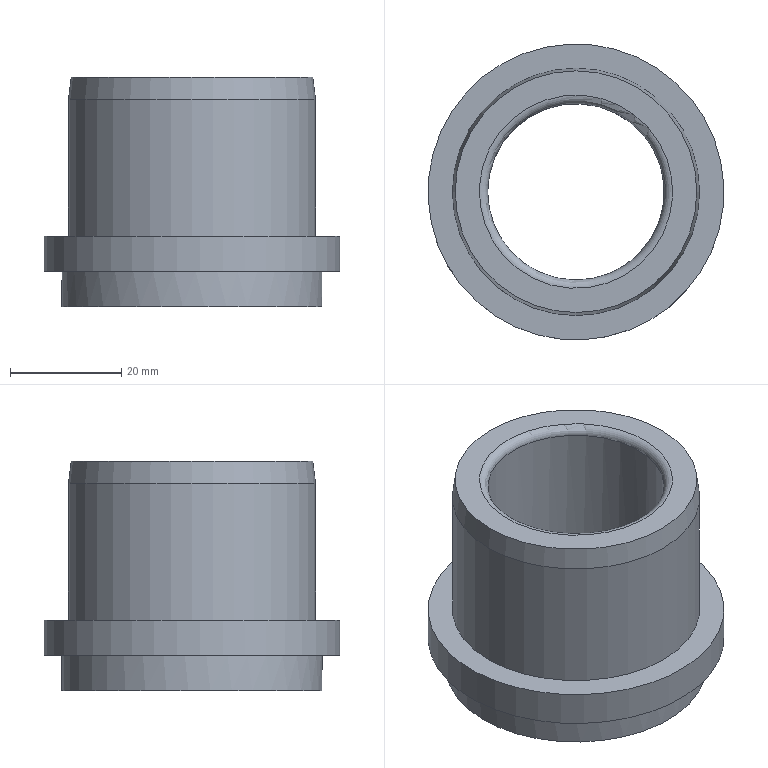Part | STEP file | 1_id1062_x_t | 1 solid | 11 faces | box 53.213 x 53.213 x 41.275 mm | volume 36326 mm3 | plane 4 | cylinder 4 | torus 2 | cone 1 | commonest cylinder face diameters 31.75 x1 44.45 x1 46.812 x1 53.213 x1
STEP:
#1=CARTESIAN_POINT('',(0.,0.,0.));
#2=DIRECTION('',(0.,0.,1.));
#3=DIRECTION('',(1.,0.,0.));
#4=AXIS2_PLACEMENT_3D('',#1,#2,#3);
#5=CARTESIAN_POINT('',(881.739,298.363,118.685));
#6=VERTEX_POINT('',#5);
#7=CARTESIAN_POINT('',(862.925,287.5,118.685));
#8=DIRECTION('',(0.,0.,1.));
#9=DIRECTION('',(0.866,0.5,0.));
#10=AXIS2_PLACEMENT_3D('',#7,#8,#9);
#11=CIRCLE('',#10,21.725);
#12=CARTESIAN_POINT('',(845.604,277.5,118.685));
#13=DIRECTION('',(0.,0.,1.));
#14=DIRECTION('',(-0.866,-0.5,0.));
#15=AXIS2_PLACEMENT_3D('',#12,#13,#14);
#16=PLANE('',#15);
#17=CARTESIAN_POINT('',(-20.,0.));
#18=DIRECTION('',(-1.,0.));
#19=AXIS2_PLACEMENT_2D('',#17,#18);
#20=CIRCLE('',#19,21.725);
#21=(GEOMETRIC_REPRESENTATION_CONTEXT(2)PARAMETRIC_REPRESENTATION_CONTEXT()REPRESENTATION_CONTEXT('',''));
#22=DEFINITIONAL_REPRESENTATION('',(#20),#21);
#23=PCURVE('',#16,#22);
#24=CARTESIAN_POINT('',(862.925,287.5,116.685));
#25=DIRECTION('',(0.,0.,-1.));
#26=DIRECTION('',(0.866,0.5,0.));
#27=AXIS2_PLACEMENT_3D('',#24,#25,#26);
#28=CONICAL_SURFACE('',#27,21.975,0.1244);
#29=CARTESIAN_POINT('',(6.283,-2.));
#30=DIRECTION('',(-1.,0.));
#31=VECTOR('',#30,1.);
#32=LINE('',#29,#31);
#33=(GEOMETRIC_REPRESENTATION_CONTEXT(2)PARAMETRIC_REPRESENTATION_CONTEXT()REPRESENTATION_CONTEXT('',''));
#34=DEFINITIONAL_REPRESENTATION('',(#32),#33);
#35=PCURVE('',#28,#34);
#36=SURFACE_CURVE('',#11,(#23,#35),.PCURVE_S1.);
#37=EDGE_CURVE('',#6,#6,#36,.T.);
#38=ORIENTED_EDGE('',*,*,#37,.T.);
#39=EDGE_LOOP('',(#38));
#40=FACE_BOUND('',#39,.T.);
#41=CARTESIAN_POINT('',(877.972,296.188,118.685));
#42=VERTEX_POINT('',#41);
#43=CARTESIAN_POINT('',(847.878,278.812,118.685));
#44=VERTEX_POINT('',#43);
#45=CARTESIAN_POINT('',(862.925,287.5,118.685));
#46=DIRECTION('',(0.,0.,-1.));
#47=DIRECTION('',(0.866,0.5,0.));
#48=AXIS2_PLACEMENT_3D('',#45,#46,#47);
#49=CIRCLE('',#48,17.375);
#50=CARTESIAN_POINT('',(-37.375,0.));
#51=CARTESIAN_POINT('',(-37.375,30.094));
#52=CARTESIAN_POINT('',(-11.313,15.047));
#53=CARTESIAN_POINT('',(14.75,0.));
#54=CARTESIAN_POINT('',(-11.313,-15.047));
#55=CARTESIAN_POINT('',(-37.375,-30.094));
#56=CARTESIAN_POINT('',(-37.375,0.));
#57=(BOUNDED_CURVE()B_SPLINE_CURVE(2,(#50,#51,#52,#53,#54,#55,#56),.UNSPECIFIED.,.T.,.F.)B_SPLINE_CURVE_WITH_KNOTS((1,2,2,2,2,1),(-2.094,0.,2.094,4.189,6.283,8.378),.UNSPECIFIED.)CURVE()GEOMETRIC_REPRESENTATION_ITEM()RATIONAL_B_SPLINE_CURVE((1.,0.5,1.,0.5,1.,0.5,1.))REPRESENTATION_ITEM(''));
#58=(GEOMETRIC_REPRESENTATION_CONTEXT(2)PARAMETRIC_REPRESENTATION_CONTEXT()REPRESENTATION_CONTEXT('',''));
#59=DEFINITIONAL_REPRESENTATION('',(#57),#58);
#60=PCURVE('',#16,#59);
#61=CARTESIAN_POINT('',(862.925,287.5,117.185));
#62=DIRECTION('',(0.,0.,1.));
#63=DIRECTION('',(-0.866,-0.5,0.));
#64=AXIS2_PLACEMENT_3D('',#61,#62,#63);
#65=TOROIDAL_SURFACE('',#64,17.375,1.5);
#66=CARTESIAN_POINT('',(3.142,7.854));
#67=DIRECTION('',(-1.,0.));
#68=VECTOR('',#67,1.);
#69=LINE('',#66,#68);
#70=(GEOMETRIC_REPRESENTATION_CONTEXT(2)PARAMETRIC_REPRESENTATION_CONTEXT()REPRESENTATION_CONTEXT('',''));
#71=DEFINITIONAL_REPRESENTATION('',(#69),#70);
#72=PCURVE('',#65,#71);
#73=SURFACE_CURVE('',#49,(#60,#72),.PCURVE_S1.);
#74=EDGE_CURVE('',#42,#44,#73,.T.);
#75=ORIENTED_EDGE('',*,*,#74,.T.);
#76=CARTESIAN_POINT('',(862.925,287.5,118.685));
#77=DIRECTION('',(0.,0.,-1.));
#78=DIRECTION('',(0.866,0.5,0.));
#79=AXIS2_PLACEMENT_3D('',#76,#77,#78);
#80=CIRCLE('',#79,17.375);
#81=CARTESIAN_POINT('',(-37.375,0.));
#82=CARTESIAN_POINT('',(-37.375,30.094));
#83=CARTESIAN_POINT('',(-11.313,15.047));
#84=CARTESIAN_POINT('',(14.75,0.));
#85=CARTESIAN_POINT('',(-11.313,-15.047));
#86=CARTESIAN_POINT('',(-37.375,-30.094));
#87=CARTESIAN_POINT('',(-37.375,0.));
#88=(BOUNDED_CURVE()B_SPLINE_CURVE(2,(#81,#82,#83,#84,#85,#86,#87),.UNSPECIFIED.,.T.,.F.)B_SPLINE_CURVE_WITH_KNOTS((1,2,2,2,2,1),(-2.094,0.,2.094,4.189,6.283,8.378),.UNSPECIFIED.)CURVE()GEOMETRIC_REPRESENTATION_ITEM()RATIONAL_B_SPLINE_CURVE((1.,0.5,1.,0.5,1.,0.5,1.))REPRESENTATION_ITEM(''));
#89=(GEOMETRIC_REPRESENTATION_CONTEXT(2)PARAMETRIC_REPRESENTATION_CONTEXT()REPRESENTATION_CONTEXT('',''));
#90=DEFINITIONAL_REPRESENTATION('',(#88),#89);
#91=PCURVE('',#16,#90);
#92=CARTESIAN_POINT('',(9.425,7.854));
#93=DIRECTION('',(-1.,0.));
#94=VECTOR('',#93,1.);
#95=LINE('',#92,#94);
#96=(GEOMETRIC_REPRESENTATION_CONTEXT(2)PARAMETRIC_REPRESENTATION_CONTEXT()REPRESENTATION_CONTEXT('',''));
#97=DEFINITIONAL_REPRESENTATION('',(#95),#96);
#98=PCURVE('',#65,#97);
#99=SURFACE_CURVE('',#80,(#91,#98),.PCURVE_S1.);
#100=EDGE_CURVE('',#44,#42,#99,.T.);
#101=ORIENTED_EDGE('',*,*,#100,.T.);
#102=EDGE_LOOP('',(#75,#101));
#103=FACE_BOUND('',#102,.T.);
#104=ADVANCED_FACE('',(#40,#103),#16,.T.);
#105=CARTESIAN_POINT('',(882.172,298.613,114.685));
#106=VERTEX_POINT('',#105);
#107=CARTESIAN_POINT('',(851.812,306.747,114.685));
#108=VERTEX_POINT('',#107);
#109=CARTESIAN_POINT('',(862.925,287.5,114.685));
#110=DIRECTION('',(0.,0.,1.));
#111=DIRECTION('',(0.866,0.5,0.));
#112=AXIS2_PLACEMENT_3D('',#109,#110,#111);
#113=CIRCLE('',#112,22.225);
#114=CARTESIAN_POINT('',(6.283,2.));
#115=DIRECTION('',(-1.,0.));
#116=VECTOR('',#115,1.);
#117=LINE('',#114,#116);
#118=(GEOMETRIC_REPRESENTATION_CONTEXT(2)PARAMETRIC_REPRESENTATION_CONTEXT()REPRESENTATION_CONTEXT('',''));
#119=DEFINITIONAL_REPRESENTATION('',(#117),#118);
#120=PCURVE('',#28,#119);
#121=CARTESIAN_POINT('',(862.925,287.5,72.685));
#122=DIRECTION('',(0.,0.,1.));
#123=DIRECTION('',(-0.5,0.866,0.));
#124=AXIS2_PLACEMENT_3D('',#121,#122,#123);
#125=CYLINDRICAL_SURFACE('',#124,22.225);
#126=CARTESIAN_POINT('',(4.712,42.));
#127=DIRECTION('',(1.,0.));
#128=VECTOR('',#127,1.);
#129=LINE('',#126,#128);
#130=(GEOMETRIC_REPRESENTATION_CONTEXT(2)PARAMETRIC_REPRESENTATION_CONTEXT()REPRESENTATION_CONTEXT('',''));
#131=DEFINITIONAL_REPRESENTATION('',(#129),#130);
#132=PCURVE('',#125,#131);
#133=SURFACE_CURVE('',#113,(#120,#132),.PCURVE_S1.);
#134=EDGE_CURVE('',#106,#108,#133,.T.);
#135=ORIENTED_EDGE('',*,*,#134,.T.);
#136=CARTESIAN_POINT('',(862.925,287.5,114.685));
#137=DIRECTION('',(0.,0.,1.));
#138=DIRECTION('',(0.866,0.5,0.));
#139=AXIS2_PLACEMENT_3D('',#136,#137,#138);
#140=CIRCLE('',#139,22.225);
#141=CARTESIAN_POINT('',(6.283,2.));
#142=DIRECTION('',(-1.,0.));
#143=VECTOR('',#142,1.);
#144=LINE('',#141,#143);
#145=(GEOMETRIC_REPRESENTATION_CONTEXT(2)PARAMETRIC_REPRESENTATION_CONTEXT()REPRESENTATION_CONTEXT('',''));
#146=DEFINITIONAL_REPRESENTATION('',(#144),#145);
#147=PCURVE('',#28,#146);
#148=CARTESIAN_POINT('',(-1.571,42.));
#149=DIRECTION('',(1.,0.));
#150=VECTOR('',#149,1.);
#151=LINE('',#148,#150);
#152=(GEOMETRIC_REPRESENTATION_CONTEXT(2)PARAMETRIC_REPRESENTATION_CONTEXT()REPRESENTATION_CONTEXT('',''));
#153=DEFINITIONAL_REPRESENTATION('',(#151),#152);
#154=PCURVE('',#125,#153);
#155=SURFACE_CURVE('',#140,(#147,#154),.PCURVE_S1.);
#156=EDGE_CURVE('',#108,#106,#155,.T.);
#157=ORIENTED_EDGE('',*,*,#156,.T.);
#158=CARTESIAN_POINT('',(881.739,298.363,118.685));
#159=CARTESIAN_POINT('',(882.172,298.612,114.685));
#160=B_SPLINE_CURVE_WITH_KNOTS('',1,(#158,#159),.UNSPECIFIED.,.F.,.F.,(2,2),(-2.016,2.016),.PIECEWISE_BEZIER_KNOTS.);
#161=CARTESIAN_POINT('',(0.,0.));
#162=DIRECTION('',(0.,1.));
#163=VECTOR('',#162,1.);
#164=LINE('',#161,#163);
#165=(GEOMETRIC_REPRESENTATION_CONTEXT(2)PARAMETRIC_REPRESENTATION_CONTEXT()REPRESENTATION_CONTEXT('',''));
#166=DEFINITIONAL_REPRESENTATION('',(#164),#165);
#167=PCURVE('',#28,#166);
#168=CARTESIAN_POINT('',(6.283,0.));
#169=DIRECTION('',(0.,1.));
#170=VECTOR('',#169,1.);
#171=LINE('',#168,#170);
#172=(GEOMETRIC_REPRESENTATION_CONTEXT(2)PARAMETRIC_REPRESENTATION_CONTEXT()REPRESENTATION_CONTEXT('',''));
#173=DEFINITIONAL_REPRESENTATION('',(#171),#172);
#174=PCURVE('',#28,#173);
#175=SEAM_CURVE('',#160,(#167,#174),.PCURVE_S1.);
#176=EDGE_CURVE('',#6,#106,#175,.T.);
#177=ORIENTED_EDGE('',*,*,#176,.F.);
#178=ORIENTED_EDGE('',*,*,#37,.F.);
#179=ORIENTED_EDGE('',*,*,#176,.T.);
#180=EDGE_LOOP('',(#135,#157,#177,#178,#179));
#181=FACE_BOUND('',#180,.T.);
#182=ADVANCED_FACE('',(#181),#28,.T.);
#183=ORIENTED_EDGE('',*,*,#156,.F.);
#184=CARTESIAN_POINT('',(851.812,306.747,90.11));
#185=VERTEX_POINT('',#184);
#186=CARTESIAN_POINT('',(851.812,306.747,90.11));
#187=CARTESIAN_POINT('',(851.812,306.747,114.685));
#188=B_SPLINE_CURVE_WITH_KNOTS('',1,(#186,#187),.UNSPECIFIED.,.F.,.F.,(2,2),(17.425,42.),.PIECEWISE_BEZIER_KNOTS.);
#189=CARTESIAN_POINT('',(0.,0.));
#190=DIRECTION('',(0.,1.));
#191=VECTOR('',#190,1.);
#192=LINE('',#189,#191);
#193=(GEOMETRIC_REPRESENTATION_CONTEXT(2)PARAMETRIC_REPRESENTATION_CONTEXT()REPRESENTATION_CONTEXT('',''));
#194=DEFINITIONAL_REPRESENTATION('',(#192),#193);
#195=PCURVE('',#125,#194);
#196=CARTESIAN_POINT('',(6.283,0.));
#197=DIRECTION('',(0.,1.));
#198=VECTOR('',#197,1.);
#199=LINE('',#196,#198);
#200=(GEOMETRIC_REPRESENTATION_CONTEXT(2)PARAMETRIC_REPRESENTATION_CONTEXT()REPRESENTATION_CONTEXT('',''));
#201=DEFINITIONAL_REPRESENTATION('',(#199),#200);
#202=PCURVE('',#125,#201);
#203=SEAM_CURVE('',#188,(#195,#202),.PCURVE_S1.);
#204=EDGE_CURVE('',#185,#108,#203,.T.);
#205=ORIENTED_EDGE('',*,*,#204,.F.);
#206=CARTESIAN_POINT('',(862.925,287.5,90.11));
#207=DIRECTION('',(0.,0.,-1.));
#208=DIRECTION('',(-0.5,0.866,0.));
#209=AXIS2_PLACEMENT_3D('',#206,#207,#208);
#210=CIRCLE('',#209,22.225);
#211=CARTESIAN_POINT('',(6.283,17.425));
#212=DIRECTION('',(-1.,0.));
#213=VECTOR('',#212,1.);
#214=LINE('',#211,#213);
#215=(GEOMETRIC_REPRESENTATION_CONTEXT(2)PARAMETRIC_REPRESENTATION_CONTEXT()REPRESENTATION_CONTEXT('',''));
#216=DEFINITIONAL_REPRESENTATION('',(#214),#215);
#217=PCURVE('',#125,#216);
#218=CARTESIAN_POINT('',(841.274,275.,90.11));
#219=DIRECTION('',(0.,0.,1.));
#220=DIRECTION('',(-0.866,-0.5,0.));
#221=AXIS2_PLACEMENT_3D('',#218,#219,#220);
#222=PLANE('',#221);
#223=CARTESIAN_POINT('',(-25.,-22.225));
#224=CARTESIAN_POINT('',(-63.495,-22.225));
#225=CARTESIAN_POINT('',(-44.247,11.112));
#226=CARTESIAN_POINT('',(-25.,44.45));
#227=CARTESIAN_POINT('',(-5.753,11.112));
#228=CARTESIAN_POINT('',(13.495,-22.225));
#229=CARTESIAN_POINT('',(-25.,-22.225));
#230=(BOUNDED_CURVE()B_SPLINE_CURVE(2,(#223,#224,#225,#226,#227,#228,#229),.UNSPECIFIED.,.T.,.F.)B_SPLINE_CURVE_WITH_KNOTS((1,2,2,2,2,1),(-2.094,0.,2.094,4.189,6.283,8.378),.UNSPECIFIED.)CURVE()GEOMETRIC_REPRESENTATION_ITEM()RATIONAL_B_SPLINE_CURVE((1.,0.5,1.,0.5,1.,0.5,1.))REPRESENTATION_ITEM(''));
#231=(GEOMETRIC_REPRESENTATION_CONTEXT(2)PARAMETRIC_REPRESENTATION_CONTEXT()REPRESENTATION_CONTEXT('',''));
#232=DEFINITIONAL_REPRESENTATION('',(#230),#231);
#233=PCURVE('',#222,#232);
#234=SURFACE_CURVE('',#210,(#217,#233),.PCURVE_S1.);
#235=EDGE_CURVE('',#185,#185,#234,.T.);
#236=ORIENTED_EDGE('',*,*,#235,.F.);
#237=ORIENTED_EDGE('',*,*,#204,.T.);
#238=ORIENTED_EDGE('',*,*,#134,.F.);
#239=EDGE_LOOP('',(#183,#205,#236,#237,#238));
#240=FACE_BOUND('',#239,.T.);
#241=ADVANCED_FACE('',(#240),#125,.T.);
#242=CARTESIAN_POINT('',(876.228,264.458,90.11));
#243=VERTEX_POINT('',#242);
#244=CARTESIAN_POINT('',(849.622,310.542,90.11));
#245=VERTEX_POINT('',#244);
#246=CARTESIAN_POINT('',(862.925,287.5,90.11));
#247=DIRECTION('',(0.,0.,1.));
#248=DIRECTION('',(0.5,-0.866,0.));
#249=AXIS2_PLACEMENT_3D('',#246,#247,#248);
#250=CIRCLE('',#249,26.606);
#251=CARTESIAN_POINT('',(-25.,0.));
#252=DIRECTION('',(0.,1.));
#253=AXIS2_PLACEMENT_2D('',#251,#252);
#254=CIRCLE('',#253,26.606);
#255=(GEOMETRIC_REPRESENTATION_CONTEXT(2)PARAMETRIC_REPRESENTATION_CONTEXT()REPRESENTATION_CONTEXT('',''));
#256=DEFINITIONAL_REPRESENTATION('',(#254),#255);
#257=PCURVE('',#222,#256);
#258=CARTESIAN_POINT('',(862.925,287.5,84.11));
#259=DIRECTION('',(0.,0.,1.));
#260=DIRECTION('',(-0.5,0.866,0.));
#261=AXIS2_PLACEMENT_3D('',#258,#259,#260);
#262=CYLINDRICAL_SURFACE('',#261,26.606);
#263=CARTESIAN_POINT('',(3.142,6.));
#264=DIRECTION('',(1.,0.));
#265=VECTOR('',#264,1.);
#266=LINE('',#263,#265);
#267=(GEOMETRIC_REPRESENTATION_CONTEXT(2)PARAMETRIC_REPRESENTATION_CONTEXT()REPRESENTATION_CONTEXT('',''));
#268=DEFINITIONAL_REPRESENTATION('',(#266),#267);
#269=PCURVE('',#262,#268);
#270=SURFACE_CURVE('',#250,(#257,#269),.PCURVE_S1.);
#271=EDGE_CURVE('',#243,#245,#270,.T.);
#272=ORIENTED_EDGE('',*,*,#271,.T.);
#273=CARTESIAN_POINT('',(862.925,287.5,90.11));
#274=DIRECTION('',(0.,0.,1.));
#275=DIRECTION('',(0.5,-0.866,0.));
#276=AXIS2_PLACEMENT_3D('',#273,#274,#275);
#277=CIRCLE('',#276,26.606);
#278=CARTESIAN_POINT('',(-25.,0.));
#279=DIRECTION('',(0.,1.));
#280=AXIS2_PLACEMENT_2D('',#278,#279);
#281=CIRCLE('',#280,26.606);
#282=(GEOMETRIC_REPRESENTATION_CONTEXT(2)PARAMETRIC_REPRESENTATION_CONTEXT()REPRESENTATION_CONTEXT('',''));
#283=DEFINITIONAL_REPRESENTATION('',(#281),#282);
#284=PCURVE('',#222,#283);
#285=CARTESIAN_POINT('',(-3.142,6.));
#286=DIRECTION('',(1.,0.));
#287=VECTOR('',#286,1.);
#288=LINE('',#285,#287);
#289=(GEOMETRIC_REPRESENTATION_CONTEXT(2)PARAMETRIC_REPRESENTATION_CONTEXT()REPRESENTATION_CONTEXT('',''));
#290=DEFINITIONAL_REPRESENTATION('',(#288),#289);
#291=PCURVE('',#262,#290);
#292=SURFACE_CURVE('',#277,(#284,#291),.PCURVE_S1.);
#293=EDGE_CURVE('',#245,#243,#292,.T.);
#294=ORIENTED_EDGE('',*,*,#293,.T.);
#295=EDGE_LOOP('',(#272,#294));
#296=FACE_BOUND('',#295,.T.);
#297=ORIENTED_EDGE('',*,*,#235,.T.);
#298=EDGE_LOOP('',(#297));
#299=FACE_BOUND('',#298,.T.);
#300=ADVANCED_FACE('',(#296,#299),#222,.T.);
#301=ORIENTED_EDGE('',*,*,#293,.F.);
#302=CARTESIAN_POINT('',(849.622,310.542,83.76));
#303=VERTEX_POINT('',#302);
#304=CARTESIAN_POINT('',(849.622,310.542,83.76));
#305=CARTESIAN_POINT('',(849.622,310.542,90.11));
#306=B_SPLINE_CURVE_WITH_KNOTS('',1,(#304,#305),.UNSPECIFIED.,.F.,.F.,(2,2),(-0.35,6.),.PIECEWISE_BEZIER_KNOTS.);
#307=CARTESIAN_POINT('',(0.,0.));
#308=DIRECTION('',(0.,1.));
#309=VECTOR('',#308,1.);
#310=LINE('',#307,#309);
#311=(GEOMETRIC_REPRESENTATION_CONTEXT(2)PARAMETRIC_REPRESENTATION_CONTEXT()REPRESENTATION_CONTEXT('',''));
#312=DEFINITIONAL_REPRESENTATION('',(#310),#311);
#313=PCURVE('',#262,#312);
#314=CARTESIAN_POINT('',(6.283,0.));
#315=DIRECTION('',(0.,1.));
#316=VECTOR('',#315,1.);
#317=LINE('',#314,#316);
#318=(GEOMETRIC_REPRESENTATION_CONTEXT(2)PARAMETRIC_REPRESENTATION_CONTEXT()REPRESENTATION_CONTEXT('',''));
#319=DEFINITIONAL_REPRESENTATION('',(#317),#318);
#320=PCURVE('',#262,#319);
#321=SEAM_CURVE('',#306,(#313,#320),.PCURVE_S1.);
#322=EDGE_CURVE('',#303,#245,#321,.T.);
#323=ORIENTED_EDGE('',*,*,#322,.F.);
#324=CARTESIAN_POINT('',(862.925,287.5,83.76));
#325=DIRECTION('',(0.,0.,-1.));
#326=DIRECTION('',(-0.5,0.866,0.));
#327=AXIS2_PLACEMENT_3D('',#324,#325,#326);
#328=CIRCLE('',#327,26.606);
#329=CARTESIAN_POINT('',(6.283,-0.35));
#330=DIRECTION('',(-1.,0.));
#331=VECTOR('',#330,1.);
#332=LINE('',#329,#331);
#333=(GEOMETRIC_REPRESENTATION_CONTEXT(2)PARAMETRIC_REPRESENTATION_CONTEXT()REPRESENTATION_CONTEXT('',''));
#334=DEFINITIONAL_REPRESENTATION('',(#332),#333);
#335=PCURVE('',#262,#334);
#336=CARTESIAN_POINT('',(845.604,277.5,83.76));
#337=DIRECTION('',(0.,0.,-1.));
#338=DIRECTION('',(-0.5,0.866,0.));
#339=AXIS2_PLACEMENT_3D('',#336,#337,#338);
#340=PLANE('',#339);
#341=CARTESIAN_POINT('',(0.,20.));
#342=DIRECTION('',(1.,0.));
#343=AXIS2_PLACEMENT_2D('',#341,#342);
#344=CIRCLE('',#343,26.606);
#345=(GEOMETRIC_REPRESENTATION_CONTEXT(2)PARAMETRIC_REPRESENTATION_CONTEXT()REPRESENTATION_CONTEXT('',''));
#346=DEFINITIONAL_REPRESENTATION('',(#344),#345);
#347=PCURVE('',#340,#346);
#348=SURFACE_CURVE('',#328,(#335,#347),.PCURVE_S1.);
#349=EDGE_CURVE('',#303,#303,#348,.T.);
#350=ORIENTED_EDGE('',*,*,#349,.F.);
#351=ORIENTED_EDGE('',*,*,#322,.T.);
#352=ORIENTED_EDGE('',*,*,#271,.F.);
#353=EDGE_LOOP('',(#301,#323,#350,#351,#352));
#354=FACE_BOUND('',#353,.T.);
#355=ADVANCED_FACE('',(#354),#262,.T.);
#356=ORIENTED_EDGE('',*,*,#349,.T.);
#357=EDGE_LOOP('',(#356));
#358=FACE_BOUND('',#357,.T.);
#359=CARTESIAN_POINT('',(874.628,267.23,83.76));
#360=VERTEX_POINT('',#359);
#361=CARTESIAN_POINT('',(851.222,307.77,83.76));
#362=VERTEX_POINT('',#361);
#363=CARTESIAN_POINT('',(862.925,287.5,83.76));
#364=DIRECTION('',(0.,0.,1.));
#365=DIRECTION('',(0.5,-0.866,0.));
#366=AXIS2_PLACEMENT_3D('',#363,#364,#365);
#367=CIRCLE('',#366,23.406);
#368=CARTESIAN_POINT('',(-23.406,20.));
#369=CARTESIAN_POINT('',(-23.406,60.541));
#370=CARTESIAN_POINT('',(11.703,40.27));
#371=CARTESIAN_POINT('',(46.812,20.));
#372=CARTESIAN_POINT('',(11.703,-0.2703));
#373=CARTESIAN_POINT('',(-23.406,-20.541));
#374=CARTESIAN_POINT('',(-23.406,20.));
#375=(BOUNDED_CURVE()B_SPLINE_CURVE(2,(#368,#369,#370,#371,#372,#373,#374),.UNSPECIFIED.,.T.,.F.)B_SPLINE_CURVE_WITH_KNOTS((1,2,2,2,2,1),(-2.094,0.,2.094,4.189,6.283,8.378),.UNSPECIFIED.)CURVE()GEOMETRIC_REPRESENTATION_ITEM()RATIONAL_B_SPLINE_CURVE((1.,0.5,1.,0.5,1.,0.5,1.))REPRESENTATION_ITEM(''));
#376=(GEOMETRIC_REPRESENTATION_CONTEXT(2)PARAMETRIC_REPRESENTATION_CONTEXT()REPRESENTATION_CONTEXT('',''));
#377=DEFINITIONAL_REPRESENTATION('',(#375),#376);
#378=PCURVE('',#340,#377);
#379=CARTESIAN_POINT('',(862.925,287.5,84.11));
#380=DIRECTION('',(0.,0.,1.));
#381=DIRECTION('',(-0.5,0.866,0.));
#382=AXIS2_PLACEMENT_3D('',#379,#380,#381);
#383=CYLINDRICAL_SURFACE('',#382,23.406);
#384=CARTESIAN_POINT('',(3.142,-0.35));
#385=DIRECTION('',(1.,0.));
#386=VECTOR('',#385,1.);
#387=LINE('',#384,#386);
#388=(GEOMETRIC_REPRESENTATION_CONTEXT(2)PARAMETRIC_REPRESENTATION_CONTEXT()REPRESENTATION_CONTEXT('',''));
#389=DEFINITIONAL_REPRESENTATION('',(#387),#388);
#390=PCURVE('',#383,#389);
#391=SURFACE_CURVE('',#367,(#378,#390),.PCURVE_S1.);
#392=EDGE_CURVE('',#360,#362,#391,.T.);
#393=ORIENTED_EDGE('',*,*,#392,.T.);
#394=CARTESIAN_POINT('',(862.925,287.5,83.76));
#395=DIRECTION('',(0.,0.,1.));
#396=DIRECTION('',(0.5,-0.866,0.));
#397=AXIS2_PLACEMENT_3D('',#394,#395,#396);
#398=CIRCLE('',#397,23.406);
#399=CARTESIAN_POINT('',(-23.406,20.));
#400=CARTESIAN_POINT('',(-23.406,60.541));
#401=CARTESIAN_POINT('',(11.703,40.27));
#402=CARTESIAN_POINT('',(46.812,20.));
#403=CARTESIAN_POINT('',(11.703,-0.2703));
#404=CARTESIAN_POINT('',(-23.406,-20.541));
#405=CARTESIAN_POINT('',(-23.406,20.));
#406=(BOUNDED_CURVE()B_SPLINE_CURVE(2,(#399,#400,#401,#402,#403,#404,#405),.UNSPECIFIED.,.T.,.F.)B_SPLINE_CURVE_WITH_KNOTS((1,2,2,2,2,1),(-2.094,0.,2.094,4.189,6.283,8.378),.UNSPECIFIED.)CURVE()GEOMETRIC_REPRESENTATION_ITEM()RATIONAL_B_SPLINE_CURVE((1.,0.5,1.,0.5,1.,0.5,1.))REPRESENTATION_ITEM(''));
#407=(GEOMETRIC_REPRESENTATION_CONTEXT(2)PARAMETRIC_REPRESENTATION_CONTEXT()REPRESENTATION_CONTEXT('',''));
#408=DEFINITIONAL_REPRESENTATION('',(#406),#407);
#409=PCURVE('',#340,#408);
#410=CARTESIAN_POINT('',(-3.142,-0.35));
#411=DIRECTION('',(1.,0.));
#412=VECTOR('',#411,1.);
#413=LINE('',#410,#412);
#414=(GEOMETRIC_REPRESENTATION_CONTEXT(2)PARAMETRIC_REPRESENTATION_CONTEXT()REPRESENTATION_CONTEXT('',''));
#415=DEFINITIONAL_REPRESENTATION('',(#413),#414);
#416=PCURVE('',#383,#415);
#417=SURFACE_CURVE('',#398,(#409,#416),.PCURVE_S1.);
#418=EDGE_CURVE('',#362,#360,#417,.T.);
#419=ORIENTED_EDGE('',*,*,#418,.T.);
#420=EDGE_LOOP('',(#393,#419));
#421=FACE_BOUND('',#420,.T.);
#422=ADVANCED_FACE('',(#358,#421),#340,.T.);
#423=ORIENTED_EDGE('',*,*,#418,.F.);
#424=CARTESIAN_POINT('',(851.222,307.77,77.41));
#425=VERTEX_POINT('',#424);
#426=CARTESIAN_POINT('',(851.222,307.77,77.41));
#427=CARTESIAN_POINT('',(851.222,307.77,83.76));
#428=B_SPLINE_CURVE_WITH_KNOTS('',1,(#426,#427),.UNSPECIFIED.,.F.,.F.,(2,2),(-6.7,-0.35),.PIECEWISE_BEZIER_KNOTS.);
#429=CARTESIAN_POINT('',(0.,0.));
#430=DIRECTION('',(0.,1.));
#431=VECTOR('',#430,1.);
#432=LINE('',#429,#431);
#433=(GEOMETRIC_REPRESENTATION_CONTEXT(2)PARAMETRIC_REPRESENTATION_CONTEXT()REPRESENTATION_CONTEXT('',''));
#434=DEFINITIONAL_REPRESENTATION('',(#432),#433);
#435=PCURVE('',#383,#434);
#436=CARTESIAN_POINT('',(6.283,0.));
#437=DIRECTION('',(0.,1.));
#438=VECTOR('',#437,1.);
#439=LINE('',#436,#438);
#440=(GEOMETRIC_REPRESENTATION_CONTEXT(2)PARAMETRIC_REPRESENTATION_CONTEXT()REPRESENTATION_CONTEXT('',''));
#441=DEFINITIONAL_REPRESENTATION('',(#439),#440);
#442=PCURVE('',#383,#441);
#443=SEAM_CURVE('',#428,(#435,#442),.PCURVE_S1.);
#444=EDGE_CURVE('',#425,#362,#443,.T.);
#445=ORIENTED_EDGE('',*,*,#444,.F.);
#446=CARTESIAN_POINT('',(862.925,287.5,77.41));
#447=DIRECTION('',(0.,0.,-1.));
#448=DIRECTION('',(-0.5,0.866,0.));
#449=AXIS2_PLACEMENT_3D('',#446,#447,#448);
#450=CIRCLE('',#449,23.406);
#451=CARTESIAN_POINT('',(6.283,-6.7));
#452=DIRECTION('',(-1.,0.));
#453=VECTOR('',#452,1.);
#454=LINE('',#451,#453);
#455=(GEOMETRIC_REPRESENTATION_CONTEXT(2)PARAMETRIC_REPRESENTATION_CONTEXT()REPRESENTATION_CONTEXT('',''));
#456=DEFINITIONAL_REPRESENTATION('',(#454),#455);
#457=PCURVE('',#383,#456);
#458=CARTESIAN_POINT('',(849.069,279.5,77.41));
#459=DIRECTION('',(0.,0.,-1.));
#460=DIRECTION('',(-0.5,0.866,0.));
#461=AXIS2_PLACEMENT_3D('',#458,#459,#460);
#462=PLANE('',#461);
#463=CARTESIAN_POINT('',(0.,16.));
#464=DIRECTION('',(1.,0.));
#465=AXIS2_PLACEMENT_2D('',#463,#464);
#466=CIRCLE('',#465,23.406);
#467=(GEOMETRIC_REPRESENTATION_CONTEXT(2)PARAMETRIC_REPRESENTATION_CONTEXT()REPRESENTATION_CONTEXT('',''));
#468=DEFINITIONAL_REPRESENTATION('',(#466),#467);
#469=PCURVE('',#462,#468);
#470=SURFACE_CURVE('',#450,(#457,#469),.PCURVE_S1.);
#471=EDGE_CURVE('',#425,#425,#470,.T.);
#472=ORIENTED_EDGE('',*,*,#471,.F.);
#473=ORIENTED_EDGE('',*,*,#444,.T.);
#474=ORIENTED_EDGE('',*,*,#392,.F.);
#475=EDGE_LOOP('',(#423,#445,#472,#473,#474));
#476=FACE_BOUND('',#475,.T.);
#477=ADVANCED_FACE('',(#476),#383,.T.);
#478=ORIENTED_EDGE('',*,*,#471,.T.);
#479=EDGE_LOOP('',(#478));
#480=FACE_BOUND('',#479,.T.);
#481=CARTESIAN_POINT('',(846.579,278.062,77.41));
#482=VERTEX_POINT('',#481);
#483=CARTESIAN_POINT('',(844.05,287.5,77.41));
#484=VERTEX_POINT('',#483);
#485=CARTESIAN_POINT('',(862.925,287.5,77.41));
#486=DIRECTION('',(0.,0.,1.));
#487=DIRECTION('',(-0.866,-0.5,0.));
#488=AXIS2_PLACEMENT_3D('',#485,#486,#487);
#489=CIRCLE('',#488,18.875);
#490=CARTESIAN_POINT('',(0.,-2.875));
#491=CARTESIAN_POINT('',(-32.692,-2.875));
#492=CARTESIAN_POINT('',(-16.346,25.438));
#493=CARTESIAN_POINT('',(0.,53.75));
#494=CARTESIAN_POINT('',(16.346,25.438));
#495=CARTESIAN_POINT('',(32.692,-2.875));
#496=CARTESIAN_POINT('',(0.,-2.875));
#497=(BOUNDED_CURVE()B_SPLINE_CURVE(2,(#490,#491,#492,#493,#494,#495,#496),.UNSPECIFIED.,.T.,.F.)B_SPLINE_CURVE_WITH_KNOTS((1,2,2,2,2,1),(-2.094,0.,2.094,4.189,6.283,8.378),.UNSPECIFIED.)CURVE()GEOMETRIC_REPRESENTATION_ITEM()RATIONAL_B_SPLINE_CURVE((1.,0.5,1.,0.5,1.,0.5,1.))REPRESENTATION_ITEM(''));
#498=(GEOMETRIC_REPRESENTATION_CONTEXT(2)PARAMETRIC_REPRESENTATION_CONTEXT()REPRESENTATION_CONTEXT('',''));
#499=DEFINITIONAL_REPRESENTATION('',(#497),#498);
#500=PCURVE('',#462,#499);
#501=CARTESIAN_POINT('',(862.925,287.5,80.41));
#502=DIRECTION('',(0.,0.,-1.));
#503=DIRECTION('',(0.866,0.5,0.));
#504=AXIS2_PLACEMENT_3D('',#501,#502,#503);
#505=TOROIDAL_SURFACE('',#504,18.875,3.);
#506=CARTESIAN_POINT('',(9.425,7.854));
#507=DIRECTION('',(-1.,0.));
#508=VECTOR('',#507,1.);
#509=LINE('',#506,#508);
#510=(GEOMETRIC_REPRESENTATION_CONTEXT(2)PARAMETRIC_REPRESENTATION_CONTEXT()REPRESENTATION_CONTEXT('',''));
#511=DEFINITIONAL_REPRESENTATION('',(#509),#510);
#512=PCURVE('',#505,#511);
#513=SURFACE_CURVE('',#489,(#500,#512),.PCURVE_S1.);
#514=EDGE_CURVE('',#482,#484,#513,.T.);
#515=ORIENTED_EDGE('',*,*,#514,.T.);
#516=CARTESIAN_POINT('',(862.925,287.5,77.41));
#517=DIRECTION('',(0.,0.,1.));
#518=DIRECTION('',(-0.866,-0.5,0.));
#519=AXIS2_PLACEMENT_3D('',#516,#517,#518);
#520=CIRCLE('',#519,18.875);
#521=CARTESIAN_POINT('',(0.,-2.875));
#522=CARTESIAN_POINT('',(-32.692,-2.875));
#523=CARTESIAN_POINT('',(-16.346,25.438));
#524=CARTESIAN_POINT('',(0.,53.75));
#525=CARTESIAN_POINT('',(16.346,25.438));
#526=CARTESIAN_POINT('',(32.692,-2.875));
#527=CARTESIAN_POINT('',(0.,-2.875));
#528=(BOUNDED_CURVE()B_SPLINE_CURVE(2,(#521,#522,#523,#524,#525,#526,#527),.UNSPECIFIED.,.T.,.F.)B_SPLINE_CURVE_WITH_KNOTS((1,2,2,2,2,1),(-2.094,0.,2.094,4.189,6.283,8.378),.UNSPECIFIED.)CURVE()GEOMETRIC_REPRESENTATION_ITEM()RATIONAL_B_SPLINE_CURVE((1.,0.5,1.,0.5,1.,0.5,1.))REPRESENTATION_ITEM(''));
#529=(GEOMETRIC_REPRESENTATION_CONTEXT(2)PARAMETRIC_REPRESENTATION_CONTEXT()REPRESENTATION_CONTEXT('',''));
#530=DEFINITIONAL_REPRESENTATION('',(#528),#529);
#531=PCURVE('',#462,#530);
#532=CARTESIAN_POINT('',(15.708,7.854));
#533=DIRECTION('',(-1.,0.));
#534=VECTOR('',#533,1.);
#535=LINE('',#532,#534);
#536=(GEOMETRIC_REPRESENTATION_CONTEXT(2)PARAMETRIC_REPRESENTATION_CONTEXT()REPRESENTATION_CONTEXT('',''));
#537=DEFINITIONAL_REPRESENTATION('',(#535),#536);
#538=PCURVE('',#505,#537);
#539=SURFACE_CURVE('',#520,(#531,#538),.PCURVE_S1.);
#540=EDGE_CURVE('',#484,#482,#539,.T.);
#541=ORIENTED_EDGE('',*,*,#540,.T.);
#542=EDGE_LOOP('',(#515,#541));
#543=FACE_BOUND('',#542,.T.);
#544=ADVANCED_FACE('',(#480,#543),#462,.T.);
#545=CARTESIAN_POINT('',(847.05,287.5,80.41));
#546=VERTEX_POINT('',#545);
#547=CARTESIAN_POINT('',(862.925,287.5,80.41));
#548=DIRECTION('',(0.,0.,1.));
#549=DIRECTION('',(-1.,0.,0.));
#550=AXIS2_PLACEMENT_3D('',#547,#548,#549);
#551=CIRCLE('',#550,15.875);
#552=CARTESIAN_POINT('',(9.948,9.425));
#553=DIRECTION('',(-1.,0.));
#554=VECTOR('',#553,1.);
#555=LINE('',#552,#554);
#556=(GEOMETRIC_REPRESENTATION_CONTEXT(2)PARAMETRIC_REPRESENTATION_CONTEXT()REPRESENTATION_CONTEXT('',''));
#557=DEFINITIONAL_REPRESENTATION('',(#555),#556);
#558=PCURVE('',#505,#557);
#559=CARTESIAN_POINT('',(862.925,287.5,72.685));
#560=DIRECTION('',(0.,0.,1.));
#561=DIRECTION('',(-0.5,0.866,0.));
#562=AXIS2_PLACEMENT_3D('',#559,#560,#561);
#563=CYLINDRICAL_SURFACE('',#562,15.875);
#564=CARTESIAN_POINT('',(1.047,7.725));
#565=DIRECTION('',(1.,0.));
#566=VECTOR('',#565,1.);
#567=LINE('',#564,#566);
#568=(GEOMETRIC_REPRESENTATION_CONTEXT(2)PARAMETRIC_REPRESENTATION_CONTEXT()REPRESENTATION_CONTEXT('',''));
#569=DEFINITIONAL_REPRESENTATION('',(#567),#568);
#570=PCURVE('',#563,#569);
#571=SURFACE_CURVE('',#551,(#558,#570),.PCURVE_S1.);
#572=EDGE_CURVE('',#546,#546,#571,.T.);
#573=ORIENTED_EDGE('',*,*,#572,.T.);
#574=CARTESIAN_POINT('',(844.05,287.5,77.41));
#575=CARTESIAN_POINT('',(844.852,287.5,77.41));
#576=CARTESIAN_POINT('',(845.633,287.5,77.665));
#577=CARTESIAN_POINT('',(846.306,287.5,78.154));
#578=CARTESIAN_POINT('',(846.795,287.5,78.827));
#579=CARTESIAN_POINT('',(847.05,287.5,79.608));
#580=CARTESIAN_POINT('',(847.05,287.5,80.41));
#581=(BOUNDED_CURVE()B_SPLINE_CURVE(6,(#574,#575,#576,#577,#578,#579,#580),.UNSPECIFIED.,.F.,.F.)B_SPLINE_CURVE_WITH_KNOTS((7,7),(1.571,3.142),.PIECEWISE_BEZIER_KNOTS.)CURVE()GEOMETRIC_REPRESENTATION_ITEM()RATIONAL_B_SPLINE_CURVE((1.031,1.01,0.9979,0.994,0.9979,1.01,1.031))REPRESENTATION_ITEM(''));
#582=CARTESIAN_POINT('',(3.665,6.283));
#583=DIRECTION('',(0.,1.));
#584=VECTOR('',#583,1.);
#585=LINE('',#582,#584);
#586=(GEOMETRIC_REPRESENTATION_CONTEXT(2)PARAMETRIC_REPRESENTATION_CONTEXT()REPRESENTATION_CONTEXT('',''));
#587=DEFINITIONAL_REPRESENTATION('',(#585),#586);
#588=PCURVE('',#505,#587);
#589=CARTESIAN_POINT('',(9.948,6.283));
#590=DIRECTION('',(0.,1.));
#591=VECTOR('',#590,1.);
#592=LINE('',#589,#591);
#593=(GEOMETRIC_REPRESENTATION_CONTEXT(2)PARAMETRIC_REPRESENTATION_CONTEXT()REPRESENTATION_CONTEXT('',''));
#594=DEFINITIONAL_REPRESENTATION('',(#592),#593);
#595=PCURVE('',#505,#594);
#596=SEAM_CURVE('',#581,(#588,#595),.PCURVE_S1.);
#597=EDGE_CURVE('',#484,#546,#596,.T.);
#598=ORIENTED_EDGE('',*,*,#597,.F.);
#599=ORIENTED_EDGE('',*,*,#514,.F.);
#600=ORIENTED_EDGE('',*,*,#540,.F.);
#601=ORIENTED_EDGE('',*,*,#597,.T.);
#602=EDGE_LOOP('',(#573,#598,#599,#600,#601));
#603=FACE_BOUND('',#602,.T.);
#604=ADVANCED_FACE('',(#603),#505,.T.);
#605=CARTESIAN_POINT('',(849.177,279.562,117.185));
#606=VERTEX_POINT('',#605);
#607=CARTESIAN_POINT('',(847.05,287.5,117.185));
#608=VERTEX_POINT('',#607);
#609=CARTESIAN_POINT('',(862.925,287.5,117.185));
#610=DIRECTION('',(0.,0.,-1.));
#611=DIRECTION('',(-0.866,-0.5,0.));
#612=AXIS2_PLACEMENT_3D('',#609,#610,#611);
#613=CIRCLE('',#612,15.875);
#614=CARTESIAN_POINT('',(1.571,44.5));
#615=DIRECTION('',(-1.,0.));
#616=VECTOR('',#615,1.);
#617=LINE('',#614,#616);
#618=(GEOMETRIC_REPRESENTATION_CONTEXT(2)PARAMETRIC_REPRESENTATION_CONTEXT()REPRESENTATION_CONTEXT('',''));
#619=DEFINITIONAL_REPRESENTATION('',(#617),#618);
#620=PCURVE('',#563,#619);
#621=CARTESIAN_POINT('',(6.283,9.425));
#622=DIRECTION('',(-1.,0.));
#623=VECTOR('',#622,1.);
#624=LINE('',#621,#623);
#625=(GEOMETRIC_REPRESENTATION_CONTEXT(2)PARAMETRIC_REPRESENTATION_CONTEXT()REPRESENTATION_CONTEXT('',''));
#626=DEFINITIONAL_REPRESENTATION('',(#624),#625);
#627=PCURVE('',#65,#626);
#628=SURFACE_CURVE('',#613,(#620,#627),.PCURVE_S1.);
#629=EDGE_CURVE('',#606,#608,#628,.T.);
#630=ORIENTED_EDGE('',*,*,#629,.T.);
#631=CARTESIAN_POINT('',(847.05,287.5,80.41));
#632=CARTESIAN_POINT('',(847.05,287.5,117.185));
#633=B_SPLINE_CURVE_WITH_KNOTS('',1,(#631,#632),.UNSPECIFIED.,.F.,.F.,(2,2),(7.725,44.5),.PIECEWISE_BEZIER_KNOTS.);
#634=CARTESIAN_POINT('',(1.047,0.));
#635=DIRECTION('',(0.,1.));
#636=VECTOR('',#635,1.);
#637=LINE('',#634,#636);
#638=(GEOMETRIC_REPRESENTATION_CONTEXT(2)PARAMETRIC_REPRESENTATION_CONTEXT()REPRESENTATION_CONTEXT('',''));
#639=DEFINITIONAL_REPRESENTATION('',(#637),#638);
#640=PCURVE('',#563,#639);
#641=CARTESIAN_POINT('',(7.33,0.));
#642=DIRECTION('',(0.,1.));
#643=VECTOR('',#642,1.);
#644=LINE('',#641,#643);
#645=(GEOMETRIC_REPRESENTATION_CONTEXT(2)PARAMETRIC_REPRESENTATION_CONTEXT()REPRESENTATION_CONTEXT('',''));
#646=DEFINITIONAL_REPRESENTATION('',(#644),#645);
#647=PCURVE('',#563,#646);
#648=SEAM_CURVE('',#633,(#640,#647),.PCURVE_S1.);
#649=EDGE_CURVE('',#546,#608,#648,.T.);
#650=ORIENTED_EDGE('',*,*,#649,.F.);
#651=ORIENTED_EDGE('',*,*,#572,.T.);
#652=ORIENTED_EDGE('',*,*,#649,.T.);
#653=CARTESIAN_POINT('',(862.925,287.5,117.185));
#654=DIRECTION('',(0.,0.,-1.));
#655=DIRECTION('',(-0.866,-0.5,0.));
#656=AXIS2_PLACEMENT_3D('',#653,#654,#655);
#657=CIRCLE('',#656,15.875);
#658=CARTESIAN_POINT('',(7.854,44.5));
#659=DIRECTION('',(-1.,0.));
#660=VECTOR('',#659,1.);
#661=LINE('',#658,#660);
#662=(GEOMETRIC_REPRESENTATION_CONTEXT(2)PARAMETRIC_REPRESENTATION_CONTEXT()REPRESENTATION_CONTEXT('',''));
#663=DEFINITIONAL_REPRESENTATION('',(#661),#662);
#664=PCURVE('',#563,#663);
#665=CARTESIAN_POINT('',(6.283,9.425));
#666=DIRECTION('',(-1.,0.));
#667=VECTOR('',#666,1.);
#668=LINE('',#665,#667);
#669=(GEOMETRIC_REPRESENTATION_CONTEXT(2)PARAMETRIC_REPRESENTATION_CONTEXT()REPRESENTATION_CONTEXT('',''));
#670=DEFINITIONAL_REPRESENTATION('',(#668),#669);
#671=PCURVE('',#65,#670);
#672=SURFACE_CURVE('',#657,(#664,#671),.PCURVE_S1.);
#673=EDGE_CURVE('',#608,#606,#672,.T.);
#674=ORIENTED_EDGE('',*,*,#673,.T.);
#675=EDGE_LOOP('',(#630,#650,#651,#652,#674));
#676=FACE_BOUND('',#675,.F.);
#677=ADVANCED_FACE('',(#676),#563,.F.);
#678=ORIENTED_EDGE('',*,*,#629,.T.);
#679=ORIENTED_EDGE('',*,*,#673,.T.);
#680=CARTESIAN_POINT('',(847.878,278.812,118.685));
#681=CARTESIAN_POINT('',(848.225,279.013,118.685));
#682=CARTESIAN_POINT('',(848.563,279.208,118.557));
#683=CARTESIAN_POINT('',(848.855,279.376,118.313));
#684=CARTESIAN_POINT('',(849.066,279.499,117.977));
#685=CARTESIAN_POINT('',(849.177,279.562,117.586));
#686=CARTESIAN_POINT('',(849.177,279.562,117.185));
#687=(BOUNDED_CURVE()B_SPLINE_CURVE(6,(#680,#681,#682,#683,#684,#685,#686),.UNSPECIFIED.,.F.,.F.)B_SPLINE_CURVE_WITH_KNOTS((7,7),(1.571,3.142),.PIECEWISE_BEZIER_KNOTS.)CURVE()GEOMETRIC_REPRESENTATION_ITEM()RATIONAL_B_SPLINE_CURVE((1.031,1.01,0.9979,0.994,0.9979,1.01,1.031))REPRESENTATION_ITEM(''));
#688=CARTESIAN_POINT('',(0.,6.283));
#689=DIRECTION('',(0.,1.));
#690=VECTOR('',#689,1.);
#691=LINE('',#688,#690);
#692=(GEOMETRIC_REPRESENTATION_CONTEXT(2)PARAMETRIC_REPRESENTATION_CONTEXT()REPRESENTATION_CONTEXT('',''));
#693=DEFINITIONAL_REPRESENTATION('',(#691),#692);
#694=PCURVE('',#65,#693);
#695=CARTESIAN_POINT('',(6.283,6.283));
#696=DIRECTION('',(0.,1.));
#697=VECTOR('',#696,1.);
#698=LINE('',#695,#697);
#699=(GEOMETRIC_REPRESENTATION_CONTEXT(2)PARAMETRIC_REPRESENTATION_CONTEXT()REPRESENTATION_CONTEXT('',''));
#700=DEFINITIONAL_REPRESENTATION('',(#698),#699);
#701=PCURVE('',#65,#700);
#702=SEAM_CURVE('',#687,(#694,#701),.PCURVE_S1.);
#703=EDGE_CURVE('',#44,#606,#702,.T.);
#704=ORIENTED_EDGE('',*,*,#703,.F.);
#705=ORIENTED_EDGE('',*,*,#74,.F.);
#706=ORIENTED_EDGE('',*,*,#100,.F.);
#707=ORIENTED_EDGE('',*,*,#703,.T.);
#708=EDGE_LOOP('',(#678,#679,#704,#705,#706,#707));
#709=FACE_BOUND('',#708,.T.);
#710=ADVANCED_FACE('',(#709),#65,.T.);
#711=CLOSED_SHELL('',(#104,#182,#241,#300,#355,#422,#477,#544,#604,#677,#710));
#712=MANIFOLD_SOLID_BREP('',#711);
#713=(LENGTH_UNIT()NAMED_UNIT(*)SI_UNIT(.MILLI.,.METRE.));
#714=UNCERTAINTY_MEASURE_WITH_UNIT(LENGTH_MEASURE(0.000005),#713,'','');
#715=(NAMED_UNIT(*)PLANE_ANGLE_UNIT()SI_UNIT($,.RADIAN.));
#716=(NAMED_UNIT(*)SI_UNIT($,.STERADIAN.)SOLID_ANGLE_UNIT());
#717=(GEOMETRIC_REPRESENTATION_CONTEXT(3)GLOBAL_UNCERTAINTY_ASSIGNED_CONTEXT((#714))GLOBAL_UNIT_ASSIGNED_CONTEXT((#713,#715,#716))REPRESENTATION_CONTEXT('',''));
#718=ADVANCED_BREP_SHAPE_REPRESENTATION('',(#4,#712),#717);